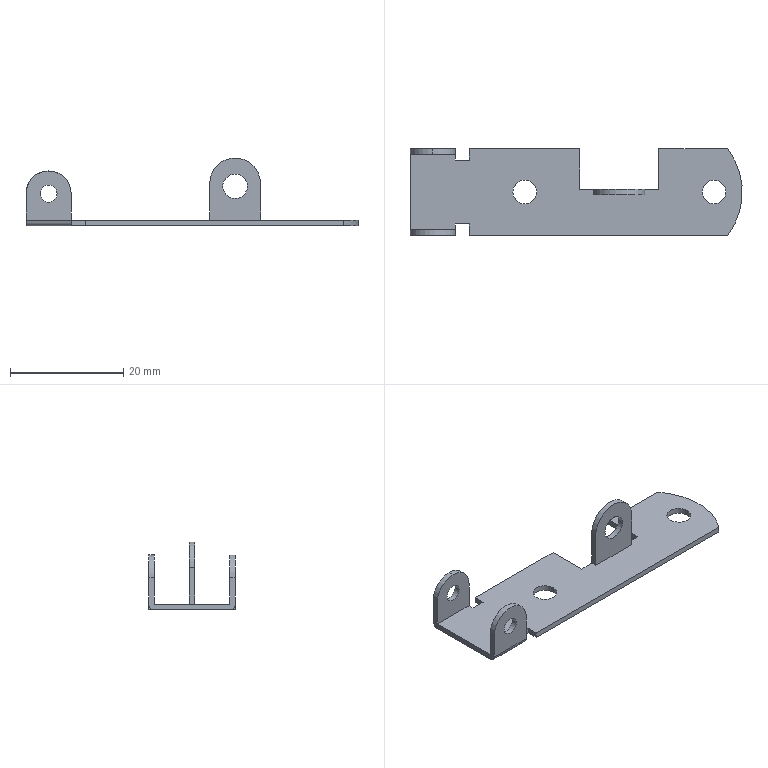Part | SolidWorks | features BaseBody 1 | 1 solid | 44 faces | box 58.8 x 15.3 x 12 mm | volume 930.521 mm3 | plane 26 | cylinder 18 | commonest cylinder face diameters 3 x4 4.2 x4 2 x3 8 x3 4.35 x2 9 x1
STEP:
#1=CARTESIAN_POINT('',(51.7,0.,0.));
#2=VERTEX_POINT('',#1);
#3=CARTESIAN_POINT('',(55.9,0.,0.));
#4=VERTEX_POINT('',#3);
#5=CARTESIAN_POINT('',(53.8,0.,0.));
#6=DIRECTION('',(0.,0.,-1.));
#7=DIRECTION('',(-1.,0.,0.));
#8=AXIS2_PLACEMENT_3D('',#5,#6,#7);
#9=CIRCLE('',#8,2.1);
#10=EDGE_CURVE('',#2,#4,#9,.T.);
#11=ORIENTED_EDGE('',*,*,#10,.F.);
#12=CARTESIAN_POINT('',(51.7,0.,-1.));
#13=VERTEX_POINT('',#12);
#14=CARTESIAN_POINT('',(51.7,0.,-0.5));
#15=DIRECTION('',(0.,0.,-1.));
#16=VECTOR('',#15,1000.);
#17=LINE('',#14,#16);
#18=EDGE_CURVE('',#2,#13,#17,.T.);
#19=ORIENTED_EDGE('',*,*,#18,.T.);
#20=CARTESIAN_POINT('',(55.9,0.,-1.));
#21=VERTEX_POINT('',#20);
#22=CARTESIAN_POINT('',(53.8,0.,-1.));
#23=DIRECTION('',(0.,0.,-1.));
#24=DIRECTION('',(1.,0.,0.));
#25=AXIS2_PLACEMENT_3D('',#22,#23,#24);
#26=CIRCLE('',#25,2.1);
#27=EDGE_CURVE('',#13,#21,#26,.T.);
#28=ORIENTED_EDGE('',*,*,#27,.T.);
#29=CARTESIAN_POINT('',(55.9,0.,-0.5));
#30=DIRECTION('',(0.,0.,-1.));
#31=VECTOR('',#30,1000.);
#32=LINE('',#29,#31);
#33=EDGE_CURVE('',#4,#21,#32,.T.);
#34=ORIENTED_EDGE('',*,*,#33,.F.);
#35=EDGE_LOOP('',(#11,#19,#28,#34));
#36=FACE_OUTER_BOUND('',#35,.T.);
#37=CARTESIAN_POINT('',(53.8,0.,-0.5));
#38=DIRECTION('',(0.,0.,-1.));
#39=DIRECTION('',(1.,0.,0.));
#40=AXIS2_PLACEMENT_3D('',#37,#38,#39);
#41=CYLINDRICAL_SURFACE('',#40,2.1);
#42=ADVANCED_FACE('',(#36),#41,.F.);
#43=CARTESIAN_POINT('',(18.2,0.,0.));
#44=VERTEX_POINT('',#43);
#45=CARTESIAN_POINT('',(22.4,0.,0.));
#46=VERTEX_POINT('',#45);
#47=CARTESIAN_POINT('',(20.3,0.,0.));
#48=DIRECTION('',(0.,0.,-1.));
#49=DIRECTION('',(-1.,0.,0.));
#50=AXIS2_PLACEMENT_3D('',#47,#48,#49);
#51=CIRCLE('',#50,2.1);
#52=EDGE_CURVE('',#44,#46,#51,.T.);
#53=ORIENTED_EDGE('',*,*,#52,.F.);
#54=CARTESIAN_POINT('',(18.2,0.,-1.));
#55=VERTEX_POINT('',#54);
#56=CARTESIAN_POINT('',(18.2,0.,-0.5));
#57=DIRECTION('',(0.,0.,-1.));
#58=VECTOR('',#57,1000.);
#59=LINE('',#56,#58);
#60=EDGE_CURVE('',#44,#55,#59,.T.);
#61=ORIENTED_EDGE('',*,*,#60,.T.);
#62=CARTESIAN_POINT('',(22.4,0.,-1.));
#63=VERTEX_POINT('',#62);
#64=CARTESIAN_POINT('',(20.3,0.,-1.));
#65=DIRECTION('',(0.,0.,-1.));
#66=DIRECTION('',(-1.,0.,0.));
#67=AXIS2_PLACEMENT_3D('',#64,#65,#66);
#68=CIRCLE('',#67,2.1);
#69=EDGE_CURVE('',#55,#63,#68,.T.);
#70=ORIENTED_EDGE('',*,*,#69,.T.);
#71=CARTESIAN_POINT('',(22.4,0.,-0.5));
#72=DIRECTION('',(0.,0.,-1.));
#73=VECTOR('',#72,1000.);
#74=LINE('',#71,#73);
#75=EDGE_CURVE('',#46,#63,#74,.T.);
#76=ORIENTED_EDGE('',*,*,#75,.F.);
#77=EDGE_LOOP('',(#53,#61,#70,#76));
#78=FACE_OUTER_BOUND('',#77,.T.);
#79=CARTESIAN_POINT('',(20.3,0.,-0.5));
#80=DIRECTION('',(0.,0.,-1.));
#81=DIRECTION('',(1.,0.,0.));
#82=AXIS2_PLACEMENT_3D('',#79,#80,#81);
#83=CYLINDRICAL_SURFACE('',#82,2.1);
#84=ADVANCED_FACE('',(#78),#83,.F.);
#85=CARTESIAN_POINT('',(34.825,0.5,6.));
#86=VERTEX_POINT('',#85);
#87=CARTESIAN_POINT('',(39.175,0.5,6.));
#88=VERTEX_POINT('',#87);
#89=CARTESIAN_POINT('',(37.,0.5,6.));
#90=DIRECTION('',(0.,-1.,0.));
#91=DIRECTION('',(-1.,0.,0.));
#92=AXIS2_PLACEMENT_3D('',#89,#90,#91);
#93=CIRCLE('',#92,2.175);
#94=EDGE_CURVE('',#86,#88,#93,.T.);
#95=ORIENTED_EDGE('',*,*,#94,.F.);
#96=CARTESIAN_POINT('',(34.825,-0.5,6.));
#97=VERTEX_POINT('',#96);
#98=CARTESIAN_POINT('',(34.825,-0.5,6.));
#99=DIRECTION('',(0.,-1.,0.));
#100=VECTOR('',#99,1000.);
#101=LINE('',#98,#100);
#102=EDGE_CURVE('',#86,#97,#101,.T.);
#103=ORIENTED_EDGE('',*,*,#102,.T.);
#104=CARTESIAN_POINT('',(39.175,-0.5,6.));
#105=VERTEX_POINT('',#104);
#106=CARTESIAN_POINT('',(37.,-0.5,6.));
#107=DIRECTION('',(0.,-1.,0.));
#108=DIRECTION('',(1.,0.,0.));
#109=AXIS2_PLACEMENT_3D('',#106,#107,#108);
#110=CIRCLE('',#109,2.175);
#111=EDGE_CURVE('',#97,#105,#110,.T.);
#112=ORIENTED_EDGE('',*,*,#111,.T.);
#113=CARTESIAN_POINT('',(39.175,-0.5,6.));
#114=DIRECTION('',(0.,-1.,0.));
#115=VECTOR('',#114,1000.);
#116=LINE('',#113,#115);
#117=EDGE_CURVE('',#88,#105,#116,.T.);
#118=ORIENTED_EDGE('',*,*,#117,.F.);
#119=EDGE_LOOP('',(#95,#103,#112,#118));
#120=FACE_OUTER_BOUND('',#119,.T.);
#121=CARTESIAN_POINT('',(37.,-0.5,6.));
#122=DIRECTION('',(0.,-1.,0.));
#123=DIRECTION('',(1.,0.,0.));
#124=AXIS2_PLACEMENT_3D('',#121,#122,#123);
#125=CYLINDRICAL_SURFACE('',#124,2.175);
#126=ADVANCED_FACE('',(#120),#125,.F.);
#127=CARTESIAN_POINT('',(0.,6.65,4.7));
#128=VERTEX_POINT('',#127);
#129=CARTESIAN_POINT('',(4.,6.65,8.7));
#130=VERTEX_POINT('',#129);
#131=CARTESIAN_POINT('',(4.,6.65,4.7));
#132=DIRECTION('',(0.,1.,0.));
#133=DIRECTION('',(-1.,0.,0.));
#134=AXIS2_PLACEMENT_3D('',#131,#132,#133);
#135=CIRCLE('',#134,4.);
#136=EDGE_CURVE('',#128,#130,#135,.T.);
#137=ORIENTED_EDGE('',*,*,#136,.T.);
#138=CARTESIAN_POINT('',(4.,7.65,8.7));
#139=VERTEX_POINT('',#138);
#140=CARTESIAN_POINT('',(4.,-27.595,8.7));
#141=DIRECTION('',(0.,1.,0.));
#142=VECTOR('',#141,1000.);
#143=LINE('',#140,#142);
#144=EDGE_CURVE('',#130,#139,#143,.T.);
#145=ORIENTED_EDGE('',*,*,#144,.T.);
#146=CARTESIAN_POINT('',(0.,7.65,4.7));
#147=VERTEX_POINT('',#146);
#148=CARTESIAN_POINT('',(4.,7.65,4.7));
#149=DIRECTION('',(0.,-1.,0.));
#150=DIRECTION('',(1.,0.,0.));
#151=AXIS2_PLACEMENT_3D('',#148,#149,#150);
#152=CIRCLE('',#151,4.);
#153=EDGE_CURVE('',#139,#147,#152,.T.);
#154=ORIENTED_EDGE('',*,*,#153,.T.);
#155=CARTESIAN_POINT('',(0.,6.65,4.7));
#156=DIRECTION('',(0.,1.,0.));
#157=VECTOR('',#156,1000.);
#158=LINE('',#155,#157);
#159=EDGE_CURVE('',#128,#147,#158,.T.);
#160=ORIENTED_EDGE('',*,*,#159,.F.);
#161=EDGE_LOOP('',(#137,#145,#154,#160));
#162=FACE_OUTER_BOUND('',#161,.T.);
#163=CARTESIAN_POINT('',(4.,-27.595,4.7));
#164=DIRECTION('',(0.,1.,0.));
#165=DIRECTION('',(0.,0.,1.));
#166=AXIS2_PLACEMENT_3D('',#163,#164,#165);
#167=CYLINDRICAL_SURFACE('',#166,4.);
#168=ADVANCED_FACE('',(#162),#167,.T.);
#169=CARTESIAN_POINT('',(5.5,-6.65,4.7));
#170=VERTEX_POINT('',#169);
#171=CARTESIAN_POINT('',(2.5,-6.65,4.7));
#172=VERTEX_POINT('',#171);
#173=CARTESIAN_POINT('',(4.,-6.65,4.7));
#174=DIRECTION('',(0.,-1.,0.));
#175=DIRECTION('',(1.,0.,0.));
#176=AXIS2_PLACEMENT_3D('',#173,#174,#175);
#177=CIRCLE('',#176,1.5);
#178=EDGE_CURVE('',#170,#172,#177,.T.);
#179=ORIENTED_EDGE('',*,*,#178,.F.);
#180=CARTESIAN_POINT('',(5.5,-7.65,4.7));
#181=VERTEX_POINT('',#180);
#182=CARTESIAN_POINT('',(5.5,-7.15,4.7));
#183=DIRECTION('',(0.,-1.,0.));
#184=VECTOR('',#183,1000.);
#185=LINE('',#182,#184);
#186=EDGE_CURVE('',#170,#181,#185,.T.);
#187=ORIENTED_EDGE('',*,*,#186,.T.);
#188=CARTESIAN_POINT('',(2.5,-7.65,4.7));
#189=VERTEX_POINT('',#188);
#190=CARTESIAN_POINT('',(4.,-7.65,4.7));
#191=DIRECTION('',(0.,-1.,0.));
#192=DIRECTION('',(1.,0.,0.));
#193=AXIS2_PLACEMENT_3D('',#190,#191,#192);
#194=CIRCLE('',#193,1.5);
#195=EDGE_CURVE('',#181,#189,#194,.T.);
#196=ORIENTED_EDGE('',*,*,#195,.T.);
#197=CARTESIAN_POINT('',(2.5,-7.15,4.7));
#198=DIRECTION('',(0.,-1.,0.));
#199=VECTOR('',#198,1000.);
#200=LINE('',#197,#199);
#201=EDGE_CURVE('',#172,#189,#200,.T.);
#202=ORIENTED_EDGE('',*,*,#201,.F.);
#203=EDGE_LOOP('',(#179,#187,#196,#202));
#204=FACE_OUTER_BOUND('',#203,.T.);
#205=CARTESIAN_POINT('',(4.,-7.15,4.7));
#206=DIRECTION('',(0.,-1.,0.));
#207=DIRECTION('',(-1.,0.,0.));
#208=AXIS2_PLACEMENT_3D('',#205,#206,#207);
#209=CYLINDRICAL_SURFACE('',#208,1.5);
#210=ADVANCED_FACE('',(#204),#209,.F.);
#211=CARTESIAN_POINT('',(5.5,7.65,4.7));
#212=VERTEX_POINT('',#211);
#213=CARTESIAN_POINT('',(2.5,7.65,4.7));
#214=VERTEX_POINT('',#213);
#215=CARTESIAN_POINT('',(4.,7.65,4.7));
#216=DIRECTION('',(0.,-1.,0.));
#217=DIRECTION('',(1.,0.,0.));
#218=AXIS2_PLACEMENT_3D('',#215,#216,#217);
#219=CIRCLE('',#218,1.5);
#220=EDGE_CURVE('',#212,#214,#219,.T.);
#221=ORIENTED_EDGE('',*,*,#220,.F.);
#222=CARTESIAN_POINT('',(5.5,6.65,4.7));
#223=VERTEX_POINT('',#222);
#224=CARTESIAN_POINT('',(5.5,7.15,4.7));
#225=DIRECTION('',(0.,-1.,0.));
#226=VECTOR('',#225,1000.);
#227=LINE('',#224,#226);
#228=EDGE_CURVE('',#212,#223,#227,.T.);
#229=ORIENTED_EDGE('',*,*,#228,.T.);
#230=CARTESIAN_POINT('',(2.5,6.65,4.7));
#231=VERTEX_POINT('',#230);
#232=CARTESIAN_POINT('',(4.,6.65,4.7));
#233=DIRECTION('',(0.,-1.,0.));
#234=DIRECTION('',(1.,0.,0.));
#235=AXIS2_PLACEMENT_3D('',#232,#233,#234);
#236=CIRCLE('',#235,1.5);
#237=EDGE_CURVE('',#223,#231,#236,.T.);
#238=ORIENTED_EDGE('',*,*,#237,.T.);
#239=CARTESIAN_POINT('',(2.5,7.15,4.7));
#240=DIRECTION('',(0.,-1.,0.));
#241=VECTOR('',#240,1000.);
#242=LINE('',#239,#241);
#243=EDGE_CURVE('',#214,#231,#242,.T.);
#244=ORIENTED_EDGE('',*,*,#243,.F.);
#245=EDGE_LOOP('',(#221,#229,#238,#244));
#246=FACE_OUTER_BOUND('',#245,.T.);
#247=CARTESIAN_POINT('',(4.,7.15,4.7));
#248=DIRECTION('',(0.,-1.,0.));
#249=DIRECTION('',(-1.,0.,0.));
#250=AXIS2_PLACEMENT_3D('',#247,#248,#249);
#251=CYLINDRICAL_SURFACE('',#250,1.5);
#252=ADVANCED_FACE('',(#246),#251,.F.);
#253=ORIENTED_EDGE('',*,*,#228,.F.);
#254=CARTESIAN_POINT('',(4.,7.65,4.7));
#255=DIRECTION('',(0.,-1.,0.));
#256=DIRECTION('',(1.,0.,0.));
#257=AXIS2_PLACEMENT_3D('',#254,#255,#256);
#258=CIRCLE('',#257,1.5);
#259=EDGE_CURVE('',#214,#212,#258,.T.);
#260=ORIENTED_EDGE('',*,*,#259,.F.);
#261=ORIENTED_EDGE('',*,*,#243,.T.);
#262=CARTESIAN_POINT('',(4.,6.65,4.7));
#263=DIRECTION('',(0.,-1.,0.));
#264=DIRECTION('',(1.,0.,0.));
#265=AXIS2_PLACEMENT_3D('',#262,#263,#264);
#266=CIRCLE('',#265,1.5);
#267=EDGE_CURVE('',#231,#223,#266,.T.);
#268=ORIENTED_EDGE('',*,*,#267,.T.);
#269=EDGE_LOOP('',(#253,#260,#261,#268));
#270=FACE_OUTER_BOUND('',#269,.T.);
#271=CARTESIAN_POINT('',(4.,7.15,4.7));
#272=DIRECTION('',(0.,-1.,0.));
#273=DIRECTION('',(-1.,0.,0.));
#274=AXIS2_PLACEMENT_3D('',#271,#272,#273);
#275=CYLINDRICAL_SURFACE('',#274,1.5);
#276=ADVANCED_FACE('',(#270),#275,.F.);
#277=ORIENTED_EDGE('',*,*,#259,.T.);
#278=ORIENTED_EDGE('',*,*,#220,.T.);
#279=EDGE_LOOP('',(#277,#278));
#280=FACE_BOUND('',#279,.T.);
#281=CARTESIAN_POINT('',(8.,7.65,4.7));
#282=VERTEX_POINT('',#281);
#283=CARTESIAN_POINT('',(8.,7.65,0.));
#284=VERTEX_POINT('',#283);
#285=CARTESIAN_POINT('',(8.,7.65,4.7));
#286=DIRECTION('',(0.,0.,-1.));
#287=VECTOR('',#286,1000.);
#288=LINE('',#285,#287);
#289=EDGE_CURVE('',#282,#284,#288,.T.);
#290=ORIENTED_EDGE('',*,*,#289,.T.);
#291=CARTESIAN_POINT('',(0.,7.65,0.));
#292=VERTEX_POINT('',#291);
#293=CARTESIAN_POINT('',(8.,7.65,0.));
#294=DIRECTION('',(-1.,0.,0.));
#295=VECTOR('',#294,1000.);
#296=LINE('',#293,#295);
#297=EDGE_CURVE('',#284,#292,#296,.T.);
#298=ORIENTED_EDGE('',*,*,#297,.T.);
#299=CARTESIAN_POINT('',(0.,7.65,0.));
#300=DIRECTION('',(0.,0.,1.));
#301=VECTOR('',#300,1000.);
#302=LINE('',#299,#301);
#303=EDGE_CURVE('',#292,#147,#302,.T.);
#304=ORIENTED_EDGE('',*,*,#303,.T.);
#305=ORIENTED_EDGE('',*,*,#153,.F.);
#306=CARTESIAN_POINT('',(4.,7.65,4.7));
#307=DIRECTION('',(0.,-1.,0.));
#308=DIRECTION('',(1.,0.,0.));
#309=AXIS2_PLACEMENT_3D('',#306,#307,#308);
#310=CIRCLE('',#309,4.);
#311=EDGE_CURVE('',#282,#139,#310,.T.);
#312=ORIENTED_EDGE('',*,*,#311,.F.);
#313=EDGE_LOOP('',(#290,#298,#304,#305,#312));
#314=FACE_OUTER_BOUND('',#313,.T.);
#315=CARTESIAN_POINT('',(0.,7.65,-1.));
#316=DIRECTION('',(0.,1.,0.));
#317=DIRECTION('',(1.,0.,0.));
#318=AXIS2_PLACEMENT_3D('',#315,#316,#317);
#319=PLANE('',#318);
#320=ADVANCED_FACE('',(#280,#314),#319,.T.);
#321=CARTESIAN_POINT('',(8.,6.65,-1.));
#322=VERTEX_POINT('',#321);
#323=CARTESIAN_POINT('',(8.,6.65,0.));
#324=DIRECTION('',(-1.,0.,0.));
#325=DIRECTION('',(0.,1.,0.));
#326=AXIS2_PLACEMENT_3D('',#323,#324,#325);
#327=CIRCLE('',#326,1.);
#328=EDGE_CURVE('',#284,#322,#327,.T.);
#329=ORIENTED_EDGE('',*,*,#328,.T.);
#330=CARTESIAN_POINT('',(0.,6.65,-1.));
#331=VERTEX_POINT('',#330);
#332=CARTESIAN_POINT('',(8.,6.65,-1.));
#333=DIRECTION('',(-1.,0.,0.));
#334=VECTOR('',#333,1000.);
#335=LINE('',#332,#334);
#336=EDGE_CURVE('',#322,#331,#335,.T.);
#337=ORIENTED_EDGE('',*,*,#336,.T.);
#338=CARTESIAN_POINT('',(0.,6.65,0.));
#339=DIRECTION('',(-1.,0.,0.));
#340=DIRECTION('',(0.,1.,0.));
#341=AXIS2_PLACEMENT_3D('',#338,#339,#340);
#342=CIRCLE('',#341,1.);
#343=EDGE_CURVE('',#292,#331,#342,.T.);
#344=ORIENTED_EDGE('',*,*,#343,.F.);
#345=ORIENTED_EDGE('',*,*,#297,.F.);
#346=EDGE_LOOP('',(#329,#337,#344,#345));
#347=FACE_OUTER_BOUND('',#346,.T.);
#348=CARTESIAN_POINT('',(8.,6.65,0.));
#349=DIRECTION('',(-1.,0.,0.));
#350=DIRECTION('',(0.,1.,0.));
#351=AXIS2_PLACEMENT_3D('',#348,#349,#350);
#352=CYLINDRICAL_SURFACE('',#351,1.);
#353=ADVANCED_FACE('',(#347),#352,.T.);
#354=CARTESIAN_POINT('',(0.,-7.65,0.));
#355=VERTEX_POINT('',#354);
#356=CARTESIAN_POINT('',(0.,-6.65,-1.));
#357=VERTEX_POINT('',#356);
#358=CARTESIAN_POINT('',(0.,-6.65,0.));
#359=DIRECTION('',(1.,0.,0.));
#360=DIRECTION('',(0.,-1.,0.));
#361=AXIS2_PLACEMENT_3D('',#358,#359,#360);
#362=CIRCLE('',#361,1.);
#363=EDGE_CURVE('',#355,#357,#362,.T.);
#364=ORIENTED_EDGE('',*,*,#363,.T.);
#365=CARTESIAN_POINT('',(8.,-6.65,-1.));
#366=VERTEX_POINT('',#365);
#367=CARTESIAN_POINT('',(0.,-6.65,-1.));
#368=DIRECTION('',(1.,0.,0.));
#369=VECTOR('',#368,1000.);
#370=LINE('',#367,#369);
#371=EDGE_CURVE('',#357,#366,#370,.T.);
#372=ORIENTED_EDGE('',*,*,#371,.T.);
#373=CARTESIAN_POINT('',(8.,-7.65,0.));
#374=VERTEX_POINT('',#373);
#375=CARTESIAN_POINT('',(8.,-6.65,0.));
#376=DIRECTION('',(1.,0.,0.));
#377=DIRECTION('',(0.,-1.,0.));
#378=AXIS2_PLACEMENT_3D('',#375,#376,#377);
#379=CIRCLE('',#378,1.);
#380=EDGE_CURVE('',#374,#366,#379,.T.);
#381=ORIENTED_EDGE('',*,*,#380,.F.);
#382=CARTESIAN_POINT('',(0.,-7.65,0.));
#383=DIRECTION('',(1.,0.,0.));
#384=VECTOR('',#383,1000.);
#385=LINE('',#382,#384);
#386=EDGE_CURVE('',#355,#374,#385,.T.);
#387=ORIENTED_EDGE('',*,*,#386,.F.);
#388=EDGE_LOOP('',(#364,#372,#381,#387));
#389=FACE_OUTER_BOUND('',#388,.T.);
#390=CARTESIAN_POINT('',(0.,-6.65,0.));
#391=DIRECTION('',(1.,0.,0.));
#392=DIRECTION('',(0.,-1.,0.));
#393=AXIS2_PLACEMENT_3D('',#390,#391,#392);
#394=CYLINDRICAL_SURFACE('',#393,1.);
#395=ADVANCED_FACE('',(#389),#394,.T.);
#396=CARTESIAN_POINT('',(44.,7.65,0.));
#397=VERTEX_POINT('',#396);
#398=CARTESIAN_POINT('',(44.,7.65,-1.));
#399=VERTEX_POINT('',#398);
#400=CARTESIAN_POINT('',(44.,7.65,0.));
#401=DIRECTION('',(0.,0.,-1.));
#402=VECTOR('',#401,1000.);
#403=LINE('',#400,#402);
#404=EDGE_CURVE('',#397,#399,#403,.T.);
#405=ORIENTED_EDGE('',*,*,#404,.T.);
#406=CARTESIAN_POINT('',(44.,0.5,-1.));
#407=VERTEX_POINT('',#406);
#408=CARTESIAN_POINT('',(44.,7.65,-1.));
#409=DIRECTION('',(0.,-1.,0.));
#410=VECTOR('',#409,1000.);
#411=LINE('',#408,#410);
#412=EDGE_CURVE('',#399,#407,#411,.T.);
#413=ORIENTED_EDGE('',*,*,#412,.T.);
#414=CARTESIAN_POINT('',(44.,0.5,0.));
#415=VERTEX_POINT('',#414);
#416=CARTESIAN_POINT('',(44.,0.5,0.));
#417=DIRECTION('',(0.,0.,-1.));
#418=VECTOR('',#417,1000.);
#419=LINE('',#416,#418);
#420=EDGE_CURVE('',#415,#407,#419,.T.);
#421=ORIENTED_EDGE('',*,*,#420,.F.);
#422=CARTESIAN_POINT('',(44.,7.65,0.));
#423=DIRECTION('',(0.,-1.,0.));
#424=VECTOR('',#423,1000.);
#425=LINE('',#422,#424);
#426=EDGE_CURVE('',#397,#415,#425,.T.);
#427=ORIENTED_EDGE('',*,*,#426,.F.);
#428=EDGE_LOOP('',(#405,#413,#421,#427));
#429=FACE_OUTER_BOUND('',#428,.T.);
#430=CARTESIAN_POINT('',(44.,4.075,-0.5));
#431=DIRECTION('',(-1.,0.,0.));
#432=DIRECTION('',(0.,0.,1.));
#433=AXIS2_PLACEMENT_3D('',#430,#431,#432);
#434=PLANE('',#433);
#435=ADVANCED_FACE('',(#429),#434,.T.);
#436=CARTESIAN_POINT('',(56.186,7.65,0.));
#437=VERTEX_POINT('',#436);
#438=CARTESIAN_POINT('',(56.186,7.65,0.));
#439=DIRECTION('',(-1.,0.,0.));
#440=VECTOR('',#439,1000.);
#441=LINE('',#438,#440);
#442=EDGE_CURVE('',#437,#397,#441,.T.);
#443=ORIENTED_EDGE('',*,*,#442,.F.);
#444=CARTESIAN_POINT('',(56.186,7.65,-1.));
#445=VERTEX_POINT('',#444);
#446=CARTESIAN_POINT('',(56.186,7.65,0.));
#447=DIRECTION('',(0.,0.,-1.));
#448=VECTOR('',#447,1000.);
#449=LINE('',#446,#448);
#450=EDGE_CURVE('',#437,#445,#449,.T.);
#451=ORIENTED_EDGE('',*,*,#450,.T.);
#452=CARTESIAN_POINT('',(56.186,7.65,-1.));
#453=DIRECTION('',(-1.,0.,0.));
#454=VECTOR('',#453,1000.);
#455=LINE('',#452,#454);
#456=EDGE_CURVE('',#445,#399,#455,.T.);
#457=ORIENTED_EDGE('',*,*,#456,.T.);
#458=ORIENTED_EDGE('',*,*,#404,.F.);
#459=EDGE_LOOP('',(#443,#451,#457,#458));
#460=FACE_OUTER_BOUND('',#459,.T.);
#461=CARTESIAN_POINT('',(28.093,7.65,-0.5));
#462=DIRECTION('',(0.,1.,0.));
#463=DIRECTION('',(1.,0.,0.));
#464=AXIS2_PLACEMENT_3D('',#461,#462,#463);
#465=PLANE('',#464);
#466=ADVANCED_FACE('',(#460),#465,.T.);
#467=CARTESIAN_POINT('',(56.186,-7.65,0.));
#468=VERTEX_POINT('',#467);
#469=CARTESIAN_POINT('',(56.186,-7.65,-1.));
#470=VERTEX_POINT('',#469);
#471=CARTESIAN_POINT('',(56.186,-7.65,0.));
#472=DIRECTION('',(0.,0.,-1.));
#473=VECTOR('',#472,1000.);
#474=LINE('',#471,#473);
#475=EDGE_CURVE('',#468,#470,#474,.T.);
#476=ORIENTED_EDGE('',*,*,#475,.T.);
#477=CARTESIAN_POINT('',(46.3,0.,-1.));
#478=DIRECTION('',(0.,0.,1.));
#479=DIRECTION('',(0.7909,-0.612,0.));
#480=AXIS2_PLACEMENT_3D('',#477,#478,#479);
#481=CIRCLE('',#480,12.5);
#482=EDGE_CURVE('',#470,#445,#481,.T.);
#483=ORIENTED_EDGE('',*,*,#482,.T.);
#484=ORIENTED_EDGE('',*,*,#450,.F.);
#485=CARTESIAN_POINT('',(46.3,0.,0.));
#486=DIRECTION('',(0.,0.,1.));
#487=DIRECTION('',(0.7909,-0.612,0.));
#488=AXIS2_PLACEMENT_3D('',#485,#486,#487);
#489=CIRCLE('',#488,12.5);
#490=EDGE_CURVE('',#468,#437,#489,.T.);
#491=ORIENTED_EDGE('',*,*,#490,.F.);
#492=EDGE_LOOP('',(#476,#483,#484,#491));
#493=FACE_OUTER_BOUND('',#492,.T.);
#494=CARTESIAN_POINT('',(46.3,0.,-0.5));
#495=DIRECTION('',(0.,0.,1.));
#496=DIRECTION('',(0.7909,-0.612,0.));
#497=AXIS2_PLACEMENT_3D('',#494,#495,#496);
#498=CYLINDRICAL_SURFACE('',#497,12.5);
#499=ADVANCED_FACE('',(#493),#498,.T.);
#500=CARTESIAN_POINT('',(10.5,-7.65,-1.));
#501=VERTEX_POINT('',#500);
#502=CARTESIAN_POINT('',(10.5,-7.65,-1.));
#503=DIRECTION('',(1.,0.,0.));
#504=VECTOR('',#503,1000.);
#505=LINE('',#502,#504);
#506=EDGE_CURVE('',#501,#470,#505,.T.);
#507=ORIENTED_EDGE('',*,*,#506,.T.);
#508=ORIENTED_EDGE('',*,*,#475,.F.);
#509=CARTESIAN_POINT('',(10.5,-7.65,0.));
#510=VERTEX_POINT('',#509);
#511=CARTESIAN_POINT('',(10.5,-7.65,0.));
#512=DIRECTION('',(1.,0.,0.));
#513=VECTOR('',#512,1000.);
#514=LINE('',#511,#513);
#515=EDGE_CURVE('',#510,#468,#514,.T.);
#516=ORIENTED_EDGE('',*,*,#515,.F.);
#517=CARTESIAN_POINT('',(10.5,-7.65,0.));
#518=DIRECTION('',(0.,0.,-1.));
#519=VECTOR('',#518,1000.);
#520=LINE('',#517,#519);
#521=EDGE_CURVE('',#510,#501,#520,.T.);
#522=ORIENTED_EDGE('',*,*,#521,.T.);
#523=EDGE_LOOP('',(#507,#508,#516,#522));
#524=FACE_OUTER_BOUND('',#523,.T.);
#525=CARTESIAN_POINT('',(28.093,-7.65,-0.5));
#526=DIRECTION('',(0.,-1.,0.));
#527=DIRECTION('',(0.,0.,-1.));
#528=AXIS2_PLACEMENT_3D('',#525,#526,#527);
#529=PLANE('',#528);
#530=ADVANCED_FACE('',(#524),#529,.T.);
#531=CARTESIAN_POINT('',(10.5,-5.65,0.));
#532=VERTEX_POINT('',#531);
#533=CARTESIAN_POINT('',(10.5,-5.65,-1.));
#534=VERTEX_POINT('',#533);
#535=CARTESIAN_POINT('',(10.5,-5.65,0.));
#536=DIRECTION('',(0.,0.,-1.));
#537=VECTOR('',#536,1000.);
#538=LINE('',#535,#537);
#539=EDGE_CURVE('',#532,#534,#538,.T.);
#540=ORIENTED_EDGE('',*,*,#539,.T.);
#541=CARTESIAN_POINT('',(10.5,-7.65,-1.));
#542=DIRECTION('',(0.,1.,0.));
#543=VECTOR('',#542,1000.);
#544=LINE('',#541,#543);
#545=EDGE_CURVE('',#501,#534,#544,.T.);
#546=ORIENTED_EDGE('',*,*,#545,.F.);
#547=ORIENTED_EDGE('',*,*,#521,.F.);
#548=CARTESIAN_POINT('',(10.5,-7.65,0.));
#549=DIRECTION('',(0.,1.,0.));
#550=VECTOR('',#549,1000.);
#551=LINE('',#548,#550);
#552=EDGE_CURVE('',#510,#532,#551,.T.);
#553=ORIENTED_EDGE('',*,*,#552,.T.);
#554=EDGE_LOOP('',(#540,#546,#547,#553));
#555=FACE_OUTER_BOUND('',#554,.T.);
#556=CARTESIAN_POINT('',(10.5,-6.65,-0.5));
#557=DIRECTION('',(1.,0.,0.));
#558=DIRECTION('',(0.,1.,0.));
#559=AXIS2_PLACEMENT_3D('',#556,#557,#558);
#560=PLANE('',#559);
#561=ADVANCED_FACE('',(#555),#560,.F.);
#562=CARTESIAN_POINT('',(8.,-5.65,0.));
#563=VERTEX_POINT('',#562);
#564=CARTESIAN_POINT('',(8.,-5.65,-1.));
#565=VERTEX_POINT('',#564);
#566=CARTESIAN_POINT('',(8.,-5.65,0.));
#567=DIRECTION('',(0.,0.,-1.));
#568=VECTOR('',#567,1000.);
#569=LINE('',#566,#568);
#570=EDGE_CURVE('',#563,#565,#569,.T.);
#571=ORIENTED_EDGE('',*,*,#570,.T.);
#572=CARTESIAN_POINT('',(10.5,-5.65,-1.));
#573=DIRECTION('',(-1.,0.,0.));
#574=VECTOR('',#573,1000.);
#575=LINE('',#572,#574);
#576=EDGE_CURVE('',#534,#565,#575,.T.);
#577=ORIENTED_EDGE('',*,*,#576,.F.);
#578=ORIENTED_EDGE('',*,*,#539,.F.);
#579=CARTESIAN_POINT('',(10.5,-5.65,0.));
#580=DIRECTION('',(-1.,0.,0.));
#581=VECTOR('',#580,1000.);
#582=LINE('',#579,#581);
#583=EDGE_CURVE('',#532,#563,#582,.T.);
#584=ORIENTED_EDGE('',*,*,#583,.T.);
#585=EDGE_LOOP('',(#571,#577,#578,#584));
#586=FACE_OUTER_BOUND('',#585,.T.);
#587=CARTESIAN_POINT('',(9.25,-5.65,-0.5));
#588=DIRECTION('',(0.,1.,0.));
#589=DIRECTION('',(1.,0.,0.));
#590=AXIS2_PLACEMENT_3D('',#587,#588,#589);
#591=PLANE('',#590);
#592=ADVANCED_FACE('',(#586),#591,.F.);
#593=ORIENTED_EDGE('',*,*,#186,.F.);
#594=CARTESIAN_POINT('',(4.,-6.65,4.7));
#595=DIRECTION('',(0.,-1.,0.));
#596=DIRECTION('',(1.,0.,0.));
#597=AXIS2_PLACEMENT_3D('',#594,#595,#596);
#598=CIRCLE('',#597,1.5);
#599=EDGE_CURVE('',#172,#170,#598,.T.);
#600=ORIENTED_EDGE('',*,*,#599,.F.);
#601=ORIENTED_EDGE('',*,*,#201,.T.);
#602=CARTESIAN_POINT('',(4.,-7.65,4.7));
#603=DIRECTION('',(0.,-1.,0.));
#604=DIRECTION('',(1.,0.,0.));
#605=AXIS2_PLACEMENT_3D('',#602,#603,#604);
#606=CIRCLE('',#605,1.5);
#607=EDGE_CURVE('',#189,#181,#606,.T.);
#608=ORIENTED_EDGE('',*,*,#607,.T.);
#609=EDGE_LOOP('',(#593,#600,#601,#608));
#610=FACE_OUTER_BOUND('',#609,.T.);
#611=CARTESIAN_POINT('',(4.,-7.15,4.7));
#612=DIRECTION('',(0.,-1.,0.));
#613=DIRECTION('',(-1.,0.,0.));
#614=AXIS2_PLACEMENT_3D('',#611,#612,#613);
#615=CYLINDRICAL_SURFACE('',#614,1.5);
#616=ADVANCED_FACE('',(#610),#615,.F.);
#617=ORIENTED_EDGE('',*,*,#599,.T.);
#618=ORIENTED_EDGE('',*,*,#178,.T.);
#619=EDGE_LOOP('',(#617,#618));
#620=FACE_BOUND('',#619,.T.);
#621=CARTESIAN_POINT('',(0.,-6.65,4.7));
#622=VERTEX_POINT('',#621);
#623=CARTESIAN_POINT('',(0.,-6.65,0.));
#624=VERTEX_POINT('',#623);
#625=CARTESIAN_POINT('',(0.,-6.65,4.7));
#626=DIRECTION('',(0.,0.,-1.));
#627=VECTOR('',#626,1000.);
#628=LINE('',#625,#627);
#629=EDGE_CURVE('',#622,#624,#628,.T.);
#630=ORIENTED_EDGE('',*,*,#629,.F.);
#631=CARTESIAN_POINT('',(8.,-6.65,4.7));
#632=VERTEX_POINT('',#631);
#633=CARTESIAN_POINT('',(4.,-6.65,4.7));
#634=DIRECTION('',(0.,-1.,0.));
#635=DIRECTION('',(1.,0.,0.));
#636=AXIS2_PLACEMENT_3D('',#633,#634,#635);
#637=CIRCLE('',#636,4.);
#638=EDGE_CURVE('',#632,#622,#637,.T.);
#639=ORIENTED_EDGE('',*,*,#638,.F.);
#640=CARTESIAN_POINT('',(8.,-6.65,0.));
#641=VERTEX_POINT('',#640);
#642=CARTESIAN_POINT('',(8.,-6.65,0.));
#643=DIRECTION('',(0.,0.,1.));
#644=VECTOR('',#643,1000.);
#645=LINE('',#642,#644);
#646=EDGE_CURVE('',#641,#632,#645,.T.);
#647=ORIENTED_EDGE('',*,*,#646,.F.);
#648=CARTESIAN_POINT('',(0.,-6.65,0.));
#649=DIRECTION('',(1.,0.,0.));
#650=VECTOR('',#649,1000.);
#651=LINE('',#648,#650);
#652=EDGE_CURVE('',#624,#641,#651,.T.);
#653=ORIENTED_EDGE('',*,*,#652,.F.);
#654=EDGE_LOOP('',(#630,#639,#647,#653));
#655=FACE_OUTER_BOUND('',#654,.T.);
#656=CARTESIAN_POINT('',(8.,-6.65,-1.));
#657=DIRECTION('',(0.,-1.,0.));
#658=DIRECTION('',(0.,0.,-1.));
#659=AXIS2_PLACEMENT_3D('',#656,#657,#658);
#660=PLANE('',#659);
#661=ADVANCED_FACE('',(#620,#655),#660,.F.);
#662=CARTESIAN_POINT('',(8.,-7.65,4.7));
#663=VERTEX_POINT('',#662);
#664=CARTESIAN_POINT('',(8.,-7.65,0.));
#665=DIRECTION('',(0.,0.,1.));
#666=VECTOR('',#665,1000.);
#667=LINE('',#664,#666);
#668=EDGE_CURVE('',#374,#663,#667,.T.);
#669=ORIENTED_EDGE('',*,*,#668,.F.);
#670=ORIENTED_EDGE('',*,*,#380,.T.);
#671=CARTESIAN_POINT('',(8.,-6.65,-1.));
#672=DIRECTION('',(0.,1.,0.));
#673=VECTOR('',#672,1000.);
#674=LINE('',#671,#673);
#675=EDGE_CURVE('',#366,#565,#674,.T.);
#676=ORIENTED_EDGE('',*,*,#675,.T.);
#677=ORIENTED_EDGE('',*,*,#570,.F.);
#678=CARTESIAN_POINT('',(8.,-6.65,0.));
#679=DIRECTION('',(0.,1.,0.));
#680=VECTOR('',#679,1000.);
#681=LINE('',#678,#680);
#682=EDGE_CURVE('',#641,#563,#681,.T.);
#683=ORIENTED_EDGE('',*,*,#682,.F.);
#684=ORIENTED_EDGE('',*,*,#646,.T.);
#685=CARTESIAN_POINT('',(8.,-6.65,4.7));
#686=DIRECTION('',(0.,-1.,0.));
#687=VECTOR('',#686,1000.);
#688=LINE('',#685,#687);
#689=EDGE_CURVE('',#632,#663,#688,.T.);
#690=ORIENTED_EDGE('',*,*,#689,.T.);
#691=EDGE_LOOP('',(#669,#670,#676,#677,#683,#684,#690));
#692=FACE_OUTER_BOUND('',#691,.T.);
#693=CARTESIAN_POINT('',(8.,-7.15,4.35));
#694=DIRECTION('',(1.,0.,0.));
#695=DIRECTION('',(0.,1.,0.));
#696=AXIS2_PLACEMENT_3D('',#693,#694,#695);
#697=PLANE('',#696);
#698=ADVANCED_FACE('',(#692),#697,.T.);
#699=ORIENTED_EDGE('',*,*,#607,.F.);
#700=ORIENTED_EDGE('',*,*,#195,.F.);
#701=EDGE_LOOP('',(#699,#700));
#702=FACE_BOUND('',#701,.T.);
#703=CARTESIAN_POINT('',(0.,-7.65,4.7));
#704=VERTEX_POINT('',#703);
#705=CARTESIAN_POINT('',(0.,-7.65,4.7));
#706=DIRECTION('',(0.,0.,-1.));
#707=VECTOR('',#706,1000.);
#708=LINE('',#705,#707);
#709=EDGE_CURVE('',#704,#355,#708,.T.);
#710=ORIENTED_EDGE('',*,*,#709,.T.);
#711=ORIENTED_EDGE('',*,*,#386,.T.);
#712=ORIENTED_EDGE('',*,*,#668,.T.);
#713=CARTESIAN_POINT('',(4.,-7.65,4.7));
#714=DIRECTION('',(0.,1.,0.));
#715=DIRECTION('',(-1.,0.,0.));
#716=AXIS2_PLACEMENT_3D('',#713,#714,#715);
#717=CIRCLE('',#716,4.);
#718=EDGE_CURVE('',#704,#663,#717,.T.);
#719=ORIENTED_EDGE('',*,*,#718,.F.);
#720=EDGE_LOOP('',(#710,#711,#712,#719));
#721=FACE_OUTER_BOUND('',#720,.T.);
#722=CARTESIAN_POINT('',(8.,-7.65,-1.));
#723=DIRECTION('',(0.,-1.,0.));
#724=DIRECTION('',(0.,0.,-1.));
#725=AXIS2_PLACEMENT_3D('',#722,#723,#724);
#726=PLANE('',#725);
#727=ADVANCED_FACE('',(#702,#721),#726,.T.);
#728=ORIENTED_EDGE('',*,*,#689,.F.);
#729=ORIENTED_EDGE('',*,*,#638,.T.);
#730=CARTESIAN_POINT('',(0.,-6.65,4.7));
#731=DIRECTION('',(0.,-1.,0.));
#732=VECTOR('',#731,1000.);
#733=LINE('',#730,#732);
#734=EDGE_CURVE('',#622,#704,#733,.T.);
#735=ORIENTED_EDGE('',*,*,#734,.T.);
#736=ORIENTED_EDGE('',*,*,#718,.T.);
#737=EDGE_LOOP('',(#728,#729,#735,#736));
#738=FACE_OUTER_BOUND('',#737,.T.);
#739=CARTESIAN_POINT('',(4.,27.595,4.7));
#740=DIRECTION('',(0.,-1.,0.));
#741=DIRECTION('',(1.,0.,0.));
#742=AXIS2_PLACEMENT_3D('',#739,#740,#741);
#743=CYLINDRICAL_SURFACE('',#742,4.);
#744=ADVANCED_FACE('',(#738),#743,.T.);
#745=ORIENTED_EDGE('',*,*,#303,.F.);
#746=ORIENTED_EDGE('',*,*,#343,.T.);
#747=CARTESIAN_POINT('',(0.,6.65,-1.));
#748=DIRECTION('',(0.,-1.,0.));
#749=VECTOR('',#748,1000.);
#750=LINE('',#747,#749);
#751=EDGE_CURVE('',#331,#357,#750,.T.);
#752=ORIENTED_EDGE('',*,*,#751,.T.);
#753=ORIENTED_EDGE('',*,*,#363,.F.);
#754=ORIENTED_EDGE('',*,*,#709,.F.);
#755=ORIENTED_EDGE('',*,*,#734,.F.);
#756=ORIENTED_EDGE('',*,*,#629,.T.);
#757=CARTESIAN_POINT('',(0.,6.65,0.));
#758=VERTEX_POINT('',#757);
#759=CARTESIAN_POINT('',(0.,6.65,0.));
#760=DIRECTION('',(0.,-1.,0.));
#761=VECTOR('',#760,1000.);
#762=LINE('',#759,#761);
#763=EDGE_CURVE('',#758,#624,#762,.T.);
#764=ORIENTED_EDGE('',*,*,#763,.F.);
#765=CARTESIAN_POINT('',(0.,6.65,0.));
#766=DIRECTION('',(0.,0.,1.));
#767=VECTOR('',#766,1000.);
#768=LINE('',#765,#767);
#769=EDGE_CURVE('',#758,#128,#768,.T.);
#770=ORIENTED_EDGE('',*,*,#769,.T.);
#771=ORIENTED_EDGE('',*,*,#159,.T.);
#772=EDGE_LOOP('',(#745,#746,#752,#753,#754,#755,#756,#764,#770,#771));
#773=FACE_OUTER_BOUND('',#772,.T.);
#774=CARTESIAN_POINT('',(0.,7.15,4.35));
#775=DIRECTION('',(-1.,0.,0.));
#776=DIRECTION('',(0.,0.,1.));
#777=AXIS2_PLACEMENT_3D('',#774,#775,#776);
#778=PLANE('',#777);
#779=ADVANCED_FACE('',(#773),#778,.T.);
#780=ORIENTED_EDGE('',*,*,#267,.F.);
#781=ORIENTED_EDGE('',*,*,#237,.F.);
#782=EDGE_LOOP('',(#780,#781));
#783=FACE_BOUND('',#782,.T.);
#784=CARTESIAN_POINT('',(8.,6.65,4.7));
#785=VERTEX_POINT('',#784);
#786=CARTESIAN_POINT('',(8.,6.65,0.));
#787=VERTEX_POINT('',#786);
#788=CARTESIAN_POINT('',(8.,6.65,4.7));
#789=DIRECTION('',(0.,0.,-1.));
#790=VECTOR('',#789,1000.);
#791=LINE('',#788,#790);
#792=EDGE_CURVE('',#785,#787,#791,.T.);
#793=ORIENTED_EDGE('',*,*,#792,.F.);
#794=CARTESIAN_POINT('',(4.,6.65,4.7));
#795=DIRECTION('',(0.,1.,0.));
#796=DIRECTION('',(-1.,0.,0.));
#797=AXIS2_PLACEMENT_3D('',#794,#795,#796);
#798=CIRCLE('',#797,4.);
#799=EDGE_CURVE('',#130,#785,#798,.T.);
#800=ORIENTED_EDGE('',*,*,#799,.F.);
#801=ORIENTED_EDGE('',*,*,#136,.F.);
#802=ORIENTED_EDGE('',*,*,#769,.F.);
#803=CARTESIAN_POINT('',(8.,6.65,0.));
#804=DIRECTION('',(-1.,0.,0.));
#805=VECTOR('',#804,1000.);
#806=LINE('',#803,#805);
#807=EDGE_CURVE('',#787,#758,#806,.T.);
#808=ORIENTED_EDGE('',*,*,#807,.F.);
#809=EDGE_LOOP('',(#793,#800,#801,#802,#808));
#810=FACE_OUTER_BOUND('',#809,.T.);
#811=CARTESIAN_POINT('',(0.,6.65,-1.));
#812=DIRECTION('',(0.,1.,0.));
#813=DIRECTION('',(1.,0.,0.));
#814=AXIS2_PLACEMENT_3D('',#811,#812,#813);
#815=PLANE('',#814);
#816=ADVANCED_FACE('',(#783,#810),#815,.F.);
#817=ORIENTED_EDGE('',*,*,#144,.F.);
#818=ORIENTED_EDGE('',*,*,#799,.T.);
#819=CARTESIAN_POINT('',(8.,6.65,4.7));
#820=DIRECTION('',(0.,1.,0.));
#821=VECTOR('',#820,1000.);
#822=LINE('',#819,#821);
#823=EDGE_CURVE('',#785,#282,#822,.T.);
#824=ORIENTED_EDGE('',*,*,#823,.T.);
#825=ORIENTED_EDGE('',*,*,#311,.T.);
#826=EDGE_LOOP('',(#817,#818,#824,#825));
#827=FACE_OUTER_BOUND('',#826,.T.);
#828=CARTESIAN_POINT('',(4.,-27.595,4.7));
#829=DIRECTION('',(0.,1.,0.));
#830=DIRECTION('',(0.,0.,1.));
#831=AXIS2_PLACEMENT_3D('',#828,#829,#830);
#832=CYLINDRICAL_SURFACE('',#831,4.);
#833=ADVANCED_FACE('',(#827),#832,.T.);
#834=CARTESIAN_POINT('',(8.,5.65,0.));
#835=VERTEX_POINT('',#834);
#836=CARTESIAN_POINT('',(8.,5.65,-1.));
#837=VERTEX_POINT('',#836);
#838=CARTESIAN_POINT('',(8.,5.65,0.));
#839=DIRECTION('',(0.,0.,-1.));
#840=VECTOR('',#839,1000.);
#841=LINE('',#838,#840);
#842=EDGE_CURVE('',#835,#837,#841,.T.);
#843=ORIENTED_EDGE('',*,*,#842,.T.);
#844=CARTESIAN_POINT('',(8.,6.65,-1.));
#845=DIRECTION('',(0.,-1.,0.));
#846=VECTOR('',#845,1000.);
#847=LINE('',#844,#846);
#848=EDGE_CURVE('',#322,#837,#847,.T.);
#849=ORIENTED_EDGE('',*,*,#848,.F.);
#850=ORIENTED_EDGE('',*,*,#328,.F.);
#851=ORIENTED_EDGE('',*,*,#289,.F.);
#852=ORIENTED_EDGE('',*,*,#823,.F.);
#853=ORIENTED_EDGE('',*,*,#792,.T.);
#854=CARTESIAN_POINT('',(8.,6.65,0.));
#855=DIRECTION('',(0.,-1.,0.));
#856=VECTOR('',#855,1000.);
#857=LINE('',#854,#856);
#858=EDGE_CURVE('',#787,#835,#857,.T.);
#859=ORIENTED_EDGE('',*,*,#858,.T.);
#860=EDGE_LOOP('',(#843,#849,#850,#851,#852,#853,#859));
#861=FACE_OUTER_BOUND('',#860,.T.);
#862=CARTESIAN_POINT('',(8.,6.65,-0.5));
#863=DIRECTION('',(-1.,0.,0.));
#864=DIRECTION('',(0.,0.,1.));
#865=AXIS2_PLACEMENT_3D('',#862,#863,#864);
#866=PLANE('',#865);
#867=ADVANCED_FACE('',(#861),#866,.F.);
#868=CARTESIAN_POINT('',(10.5,5.65,0.));
#869=VERTEX_POINT('',#868);
#870=CARTESIAN_POINT('',(10.5,5.65,-1.));
#871=VERTEX_POINT('',#870);
#872=CARTESIAN_POINT('',(10.5,5.65,0.));
#873=DIRECTION('',(0.,0.,-1.));
#874=VECTOR('',#873,1000.);
#875=LINE('',#872,#874);
#876=EDGE_CURVE('',#869,#871,#875,.T.);
#877=ORIENTED_EDGE('',*,*,#876,.T.);
#878=CARTESIAN_POINT('',(8.,5.65,-1.));
#879=DIRECTION('',(1.,0.,0.));
#880=VECTOR('',#879,1000.);
#881=LINE('',#878,#880);
#882=EDGE_CURVE('',#837,#871,#881,.T.);
#883=ORIENTED_EDGE('',*,*,#882,.F.);
#884=ORIENTED_EDGE('',*,*,#842,.F.);
#885=CARTESIAN_POINT('',(8.,5.65,0.));
#886=DIRECTION('',(1.,0.,0.));
#887=VECTOR('',#886,1000.);
#888=LINE('',#885,#887);
#889=EDGE_CURVE('',#835,#869,#888,.T.);
#890=ORIENTED_EDGE('',*,*,#889,.T.);
#891=EDGE_LOOP('',(#877,#883,#884,#890));
#892=FACE_OUTER_BOUND('',#891,.T.);
#893=CARTESIAN_POINT('',(9.25,5.65,-0.5));
#894=DIRECTION('',(0.,-1.,0.));
#895=DIRECTION('',(0.,0.,-1.));
#896=AXIS2_PLACEMENT_3D('',#893,#894,#895);
#897=PLANE('',#896);
#898=ADVANCED_FACE('',(#892),#897,.F.);
#899=CARTESIAN_POINT('',(10.5,7.65,0.));
#900=VERTEX_POINT('',#899);
#901=CARTESIAN_POINT('',(10.5,7.65,-1.));
#902=VERTEX_POINT('',#901);
#903=CARTESIAN_POINT('',(10.5,7.65,0.));
#904=DIRECTION('',(0.,0.,-1.));
#905=VECTOR('',#904,1000.);
#906=LINE('',#903,#905);
#907=EDGE_CURVE('',#900,#902,#906,.T.);
#908=ORIENTED_EDGE('',*,*,#907,.T.);
#909=CARTESIAN_POINT('',(10.5,7.65,-1.));
#910=DIRECTION('',(0.,-1.,0.));
#911=VECTOR('',#910,1000.);
#912=LINE('',#909,#911);
#913=EDGE_CURVE('',#902,#871,#912,.T.);
#914=ORIENTED_EDGE('',*,*,#913,.T.);
#915=ORIENTED_EDGE('',*,*,#876,.F.);
#916=CARTESIAN_POINT('',(10.5,7.65,0.));
#917=DIRECTION('',(0.,-1.,0.));
#918=VECTOR('',#917,1000.);
#919=LINE('',#916,#918);
#920=EDGE_CURVE('',#900,#869,#919,.T.);
#921=ORIENTED_EDGE('',*,*,#920,.F.);
#922=EDGE_LOOP('',(#908,#914,#915,#921));
#923=FACE_OUTER_BOUND('',#922,.T.);
#924=CARTESIAN_POINT('',(10.5,6.65,-0.5));
#925=DIRECTION('',(-1.,0.,0.));
#926=DIRECTION('',(0.,0.,1.));
#927=AXIS2_PLACEMENT_3D('',#924,#925,#926);
#928=PLANE('',#927);
#929=ADVANCED_FACE('',(#923),#928,.T.);
#930=CARTESIAN_POINT('',(30.,7.65,-1.));
#931=VERTEX_POINT('',#930);
#932=CARTESIAN_POINT('',(30.,7.65,-1.));
#933=DIRECTION('',(-1.,0.,0.));
#934=VECTOR('',#933,1000.);
#935=LINE('',#932,#934);
#936=EDGE_CURVE('',#931,#902,#935,.T.);
#937=ORIENTED_EDGE('',*,*,#936,.T.);
#938=ORIENTED_EDGE('',*,*,#907,.F.);
#939=CARTESIAN_POINT('',(30.,7.65,0.));
#940=VERTEX_POINT('',#939);
#941=CARTESIAN_POINT('',(30.,7.65,0.));
#942=DIRECTION('',(-1.,0.,0.));
#943=VECTOR('',#942,1000.);
#944=LINE('',#941,#943);
#945=EDGE_CURVE('',#940,#900,#944,.T.);
#946=ORIENTED_EDGE('',*,*,#945,.F.);
#947=CARTESIAN_POINT('',(30.,7.65,0.));
#948=DIRECTION('',(0.,0.,-1.));
#949=VECTOR('',#948,1000.);
#950=LINE('',#947,#949);
#951=EDGE_CURVE('',#940,#931,#950,.T.);
#952=ORIENTED_EDGE('',*,*,#951,.T.);
#953=EDGE_LOOP('',(#937,#938,#946,#952));
#954=FACE_OUTER_BOUND('',#953,.T.);
#955=CARTESIAN_POINT('',(28.093,7.65,-0.5));
#956=DIRECTION('',(0.,1.,0.));
#957=DIRECTION('',(1.,0.,0.));
#958=AXIS2_PLACEMENT_3D('',#955,#956,#957);
#959=PLANE('',#958);
#960=ADVANCED_FACE('',(#954),#959,.T.);
#961=CARTESIAN_POINT('',(30.,0.5,0.));
#962=VERTEX_POINT('',#961);
#963=CARTESIAN_POINT('',(30.,0.5,-1.));
#964=VERTEX_POINT('',#963);
#965=CARTESIAN_POINT('',(30.,0.5,0.));
#966=DIRECTION('',(0.,0.,-1.));
#967=VECTOR('',#966,1000.);
#968=LINE('',#965,#967);
#969=EDGE_CURVE('',#962,#964,#968,.T.);
#970=ORIENTED_EDGE('',*,*,#969,.T.);
#971=CARTESIAN_POINT('',(30.,7.65,-1.));
#972=DIRECTION('',(0.,-1.,0.));
#973=VECTOR('',#972,1000.);
#974=LINE('',#971,#973);
#975=EDGE_CURVE('',#931,#964,#974,.T.);
#976=ORIENTED_EDGE('',*,*,#975,.F.);
#977=ORIENTED_EDGE('',*,*,#951,.F.);
#978=CARTESIAN_POINT('',(30.,7.65,0.));
#979=DIRECTION('',(0.,-1.,0.));
#980=VECTOR('',#979,1000.);
#981=LINE('',#978,#980);
#982=EDGE_CURVE('',#940,#962,#981,.T.);
#983=ORIENTED_EDGE('',*,*,#982,.T.);
#984=EDGE_LOOP('',(#970,#976,#977,#983));
#985=FACE_OUTER_BOUND('',#984,.T.);
#986=CARTESIAN_POINT('',(30.,4.075,-0.5));
#987=DIRECTION('',(-1.,0.,0.));
#988=DIRECTION('',(0.,0.,1.));
#989=AXIS2_PLACEMENT_3D('',#986,#987,#988);
#990=PLANE('',#989);
#991=ADVANCED_FACE('',(#985),#990,.F.);
#992=CARTESIAN_POINT('',(41.5,0.5,0.));
#993=VERTEX_POINT('',#992);
#994=CARTESIAN_POINT('',(41.5,0.5,-1.));
#995=VERTEX_POINT('',#994);
#996=CARTESIAN_POINT('',(41.5,0.5,0.));
#997=DIRECTION('',(0.,0.,-1.));
#998=VECTOR('',#997,1000.);
#999=LINE('',#996,#998);
#1000=EDGE_CURVE('',#993,#995,#999,.T.);
#1001=ORIENTED_EDGE('',*,*,#1000,.T.);
#1002=CARTESIAN_POINT('',(41.5,-0.5,-1.));
#1003=VERTEX_POINT('',#1002);
#1004=CARTESIAN_POINT('',(41.5,-0.5,-1.));
#1005=DIRECTION('',(0.,1.,0.));
#1006=VECTOR('',#1005,1000.);
#1007=LINE('',#1004,#1006);
#1008=EDGE_CURVE('',#1003,#995,#1007,.T.);
#1009=ORIENTED_EDGE('',*,*,#1008,.F.);
#1010=CARTESIAN_POINT('',(41.5,-0.5,0.));
#1011=VERTEX_POINT('',#1010);
#1012=CARTESIAN_POINT('',(41.5,-0.5,-1.));
#1013=DIRECTION('',(0.,0.,1.));
#1014=VECTOR('',#1013,1000.);
#1015=LINE('',#1012,#1014);
#1016=EDGE_CURVE('',#1003,#1011,#1015,.T.);
#1017=ORIENTED_EDGE('',*,*,#1016,.T.);
#1018=CARTESIAN_POINT('',(41.5,-0.5,0.));
#1019=DIRECTION('',(0.,1.,0.));
#1020=VECTOR('',#1019,1000.);
#1021=LINE('',#1018,#1020);
#1022=EDGE_CURVE('',#1011,#993,#1021,.T.);
#1023=ORIENTED_EDGE('',*,*,#1022,.T.);
#1024=EDGE_LOOP('',(#1001,#1009,#1017,#1023));
#1025=FACE_OUTER_BOUND('',#1024,.T.);
#1026=CARTESIAN_POINT('',(41.5,0.,-0.5));
#1027=DIRECTION('',(1.,0.,0.));
#1028=DIRECTION('',(0.,1.,0.));
#1029=AXIS2_PLACEMENT_3D('',#1026,#1027,#1028);
#1030=PLANE('',#1029);
#1031=ADVANCED_FACE('',(#1025),#1030,.F.);
#1032=CARTESIAN_POINT('',(41.5,-0.5,6.5));
#1033=VERTEX_POINT('',#1032);
#1034=CARTESIAN_POINT('',(41.5,-0.5,6.5));
#1035=DIRECTION('',(0.,0.,-1.));
#1036=VECTOR('',#1035,1000.);
#1037=LINE('',#1034,#1036);
#1038=EDGE_CURVE('',#1033,#1011,#1037,.T.);
#1039=ORIENTED_EDGE('',*,*,#1038,.T.);
#1040=ORIENTED_EDGE('',*,*,#1016,.F.);
#1041=CARTESIAN_POINT('',(41.5,0.5,0.));
#1042=VERTEX_POINT('',#1041);
#1043=CARTESIAN_POINT('',(41.5,-0.5,0.));
#1044=DIRECTION('',(-1.,0.,0.));
#1045=DIRECTION('',(0.,1.,0.));
#1046=AXIS2_PLACEMENT_3D('',#1043,#1044,#1045);
#1047=CIRCLE('',#1046,1.);
#1048=EDGE_CURVE('',#1042,#1003,#1047,.T.);
#1049=ORIENTED_EDGE('',*,*,#1048,.F.);
#1050=CARTESIAN_POINT('',(41.5,0.5,6.5));
#1051=VERTEX_POINT('',#1050);
#1052=CARTESIAN_POINT('',(41.5,0.5,6.5));
#1053=DIRECTION('',(0.,0.,-1.));
#1054=VECTOR('',#1053,1000.);
#1055=LINE('',#1052,#1054);
#1056=EDGE_CURVE('',#1051,#1042,#1055,.T.);
#1057=ORIENTED_EDGE('',*,*,#1056,.F.);
#1058=CARTESIAN_POINT('',(41.5,-0.5,6.5));
#1059=DIRECTION('',(0.,1.,0.));
#1060=VECTOR('',#1059,1000.);
#1061=LINE('',#1058,#1060);
#1062=EDGE_CURVE('',#1033,#1051,#1061,.T.);
#1063=ORIENTED_EDGE('',*,*,#1062,.F.);
#1064=EDGE_LOOP('',(#1039,#1040,#1049,#1057,#1063));
#1065=FACE_OUTER_BOUND('',#1064,.T.);
#1066=CARTESIAN_POINT('',(41.5,0.,5.5));
#1067=DIRECTION('',(1.,0.,0.));
#1068=DIRECTION('',(0.,1.,0.));
#1069=AXIS2_PLACEMENT_3D('',#1066,#1067,#1068);
#1070=PLANE('',#1069);
#1071=ADVANCED_FACE('',(#1065),#1070,.T.);
#1072=CARTESIAN_POINT('',(32.5,-0.5,6.5));
#1073=VERTEX_POINT('',#1072);
#1074=CARTESIAN_POINT('',(32.5,0.5,6.5));
#1075=VERTEX_POINT('',#1074);
#1076=CARTESIAN_POINT('',(32.5,-0.5,6.5));
#1077=DIRECTION('',(0.,1.,0.));
#1078=VECTOR('',#1077,1000.);
#1079=LINE('',#1076,#1078);
#1080=EDGE_CURVE('',#1073,#1075,#1079,.T.);
#1081=ORIENTED_EDGE('',*,*,#1080,.F.);
#1082=CARTESIAN_POINT('',(37.,-0.5,6.5));
#1083=DIRECTION('',(0.,1.,0.));
#1084=DIRECTION('',(-1.,0.,0.));
#1085=AXIS2_PLACEMENT_3D('',#1082,#1083,#1084);
#1086=CIRCLE('',#1085,4.5);
#1087=EDGE_CURVE('',#1073,#1033,#1086,.T.);
#1088=ORIENTED_EDGE('',*,*,#1087,.T.);
#1089=ORIENTED_EDGE('',*,*,#1062,.T.);
#1090=CARTESIAN_POINT('',(37.,0.5,6.5));
#1091=DIRECTION('',(0.,-1.,0.));
#1092=DIRECTION('',(1.,0.,0.));
#1093=AXIS2_PLACEMENT_3D('',#1090,#1091,#1092);
#1094=CIRCLE('',#1093,4.5);
#1095=EDGE_CURVE('',#1051,#1075,#1094,.T.);
#1096=ORIENTED_EDGE('',*,*,#1095,.T.);
#1097=EDGE_LOOP('',(#1081,#1088,#1089,#1096));
#1098=FACE_OUTER_BOUND('',#1097,.T.);
#1099=CARTESIAN_POINT('',(37.,-27.595,6.5));
#1100=DIRECTION('',(0.,1.,0.));
#1101=DIRECTION('',(-1.,0.,0.));
#1102=AXIS2_PLACEMENT_3D('',#1099,#1100,#1101);
#1103=CYLINDRICAL_SURFACE('',#1102,4.5);
#1104=ADVANCED_FACE('',(#1098),#1103,.T.);
#1105=CARTESIAN_POINT('',(37.,-0.5,6.));
#1106=DIRECTION('',(0.,-1.,0.));
#1107=DIRECTION('',(1.,0.,0.));
#1108=AXIS2_PLACEMENT_3D('',#1105,#1106,#1107);
#1109=CIRCLE('',#1108,2.175);
#1110=EDGE_CURVE('',#105,#97,#1109,.T.);
#1111=ORIENTED_EDGE('',*,*,#1110,.F.);
#1112=ORIENTED_EDGE('',*,*,#111,.F.);
#1113=EDGE_LOOP('',(#1111,#1112));
#1114=FACE_BOUND('',#1113,.T.);
#1115=CARTESIAN_POINT('',(32.5,-0.5,0.));
#1116=VERTEX_POINT('',#1115);
#1117=CARTESIAN_POINT('',(32.5,-0.5,0.));
#1118=DIRECTION('',(0.,0.,1.));
#1119=VECTOR('',#1118,1000.);
#1120=LINE('',#1117,#1119);
#1121=EDGE_CURVE('',#1116,#1073,#1120,.T.);
#1122=ORIENTED_EDGE('',*,*,#1121,.F.);
#1123=CARTESIAN_POINT('',(41.5,-0.5,0.));
#1124=DIRECTION('',(-1.,0.,0.));
#1125=VECTOR('',#1124,1000.);
#1126=LINE('',#1123,#1125);
#1127=EDGE_CURVE('',#1011,#1116,#1126,.T.);
#1128=ORIENTED_EDGE('',*,*,#1127,.F.);
#1129=ORIENTED_EDGE('',*,*,#1038,.F.);
#1130=ORIENTED_EDGE('',*,*,#1087,.F.);
#1131=EDGE_LOOP('',(#1122,#1128,#1129,#1130));
#1132=FACE_OUTER_BOUND('',#1131,.T.);
#1133=CARTESIAN_POINT('',(30.,-0.5,-1.));
#1134=DIRECTION('',(0.,1.,0.));
#1135=DIRECTION('',(1.,0.,0.));
#1136=AXIS2_PLACEMENT_3D('',#1133,#1134,#1135);
#1137=PLANE('',#1136);
#1138=ADVANCED_FACE('',(#1114,#1132),#1137,.F.);
#1139=ORIENTED_EDGE('',*,*,#102,.F.);
#1140=CARTESIAN_POINT('',(37.,0.5,6.));
#1141=DIRECTION('',(0.,-1.,0.));
#1142=DIRECTION('',(-1.,0.,0.));
#1143=AXIS2_PLACEMENT_3D('',#1140,#1141,#1142);
#1144=CIRCLE('',#1143,2.175);
#1145=EDGE_CURVE('',#88,#86,#1144,.T.);
#1146=ORIENTED_EDGE('',*,*,#1145,.F.);
#1147=ORIENTED_EDGE('',*,*,#117,.T.);
#1148=ORIENTED_EDGE('',*,*,#1110,.T.);
#1149=EDGE_LOOP('',(#1139,#1146,#1147,#1148));
#1150=FACE_OUTER_BOUND('',#1149,.T.);
#1151=CARTESIAN_POINT('',(37.,-0.5,6.));
#1152=DIRECTION('',(0.,-1.,0.));
#1153=DIRECTION('',(1.,0.,0.));
#1154=AXIS2_PLACEMENT_3D('',#1151,#1152,#1153);
#1155=CYLINDRICAL_SURFACE('',#1154,2.175);
#1156=ADVANCED_FACE('',(#1150),#1155,.F.);
#1157=ORIENTED_EDGE('',*,*,#1145,.T.);
#1158=ORIENTED_EDGE('',*,*,#94,.T.);
#1159=EDGE_LOOP('',(#1157,#1158));
#1160=FACE_BOUND('',#1159,.T.);
#1161=ORIENTED_EDGE('',*,*,#1056,.T.);
#1162=CARTESIAN_POINT('',(32.5,0.5,0.));
#1163=VERTEX_POINT('',#1162);
#1164=CARTESIAN_POINT('',(41.5,0.5,0.));
#1165=DIRECTION('',(-1.,0.,0.));
#1166=VECTOR('',#1165,1000.);
#1167=LINE('',#1164,#1166);
#1168=EDGE_CURVE('',#1042,#1163,#1167,.T.);
#1169=ORIENTED_EDGE('',*,*,#1168,.T.);
#1170=CARTESIAN_POINT('',(32.5,0.5,0.));
#1171=DIRECTION('',(0.,0.,1.));
#1172=VECTOR('',#1171,1000.);
#1173=LINE('',#1170,#1172);
#1174=EDGE_CURVE('',#1163,#1075,#1173,.T.);
#1175=ORIENTED_EDGE('',*,*,#1174,.T.);
#1176=ORIENTED_EDGE('',*,*,#1095,.F.);
#1177=EDGE_LOOP('',(#1161,#1169,#1175,#1176));
#1178=FACE_OUTER_BOUND('',#1177,.T.);
#1179=CARTESIAN_POINT('',(30.,0.5,-1.));
#1180=DIRECTION('',(0.,1.,0.));
#1181=DIRECTION('',(1.,0.,0.));
#1182=AXIS2_PLACEMENT_3D('',#1179,#1180,#1181);
#1183=PLANE('',#1182);
#1184=ADVANCED_FACE('',(#1160,#1178),#1183,.T.);
#1185=ORIENTED_EDGE('',*,*,#1048,.T.);
#1186=CARTESIAN_POINT('',(32.5,-0.5,-1.));
#1187=VERTEX_POINT('',#1186);
#1188=CARTESIAN_POINT('',(41.5,-0.5,-1.));
#1189=DIRECTION('',(-1.,0.,0.));
#1190=VECTOR('',#1189,1000.);
#1191=LINE('',#1188,#1190);
#1192=EDGE_CURVE('',#1003,#1187,#1191,.T.);
#1193=ORIENTED_EDGE('',*,*,#1192,.T.);
#1194=CARTESIAN_POINT('',(32.5,-0.5,0.));
#1195=DIRECTION('',(-1.,0.,0.));
#1196=DIRECTION('',(0.,1.,0.));
#1197=AXIS2_PLACEMENT_3D('',#1194,#1195,#1196);
#1198=CIRCLE('',#1197,1.);
#1199=EDGE_CURVE('',#1163,#1187,#1198,.T.);
#1200=ORIENTED_EDGE('',*,*,#1199,.F.);
#1201=ORIENTED_EDGE('',*,*,#1168,.F.);
#1202=EDGE_LOOP('',(#1185,#1193,#1200,#1201));
#1203=FACE_OUTER_BOUND('',#1202,.T.);
#1204=CARTESIAN_POINT('',(41.5,-0.5,0.));
#1205=DIRECTION('',(-1.,0.,0.));
#1206=DIRECTION('',(0.,1.,0.));
#1207=AXIS2_PLACEMENT_3D('',#1204,#1205,#1206);
#1208=CYLINDRICAL_SURFACE('',#1207,1.);
#1209=ADVANCED_FACE('',(#1203),#1208,.T.);
#1210=CARTESIAN_POINT('',(32.5,-0.5,-1.));
#1211=DIRECTION('',(0.,0.,1.));
#1212=VECTOR('',#1211,1000.);
#1213=LINE('',#1210,#1212);
#1214=EDGE_CURVE('',#1187,#1116,#1213,.T.);
#1215=ORIENTED_EDGE('',*,*,#1214,.T.);
#1216=ORIENTED_EDGE('',*,*,#1121,.T.);
#1217=ORIENTED_EDGE('',*,*,#1080,.T.);
#1218=ORIENTED_EDGE('',*,*,#1174,.F.);
#1219=ORIENTED_EDGE('',*,*,#1199,.T.);
#1220=EDGE_LOOP('',(#1215,#1216,#1217,#1218,#1219));
#1221=FACE_OUTER_BOUND('',#1220,.T.);
#1222=CARTESIAN_POINT('',(32.5,-0.1464,-0.3536));
#1223=DIRECTION('',(1.,0.,0.));
#1224=DIRECTION('',(0.,1.,0.));
#1225=AXIS2_PLACEMENT_3D('',#1222,#1223,#1224);
#1226=PLANE('',#1225);
#1227=ADVANCED_FACE('',(#1221),#1226,.F.);
#1228=ORIENTED_EDGE('',*,*,#1214,.F.);
#1229=CARTESIAN_POINT('',(32.5,0.5,-1.));
#1230=VERTEX_POINT('',#1229);
#1231=CARTESIAN_POINT('',(32.5,-0.5,-1.));
#1232=DIRECTION('',(0.,1.,0.));
#1233=VECTOR('',#1232,1000.);
#1234=LINE('',#1231,#1233);
#1235=EDGE_CURVE('',#1187,#1230,#1234,.T.);
#1236=ORIENTED_EDGE('',*,*,#1235,.T.);
#1237=CARTESIAN_POINT('',(32.5,0.5,0.));
#1238=VERTEX_POINT('',#1237);
#1239=CARTESIAN_POINT('',(32.5,0.5,0.));
#1240=DIRECTION('',(0.,0.,-1.));
#1241=VECTOR('',#1240,1000.);
#1242=LINE('',#1239,#1241);
#1243=EDGE_CURVE('',#1238,#1230,#1242,.T.);
#1244=ORIENTED_EDGE('',*,*,#1243,.F.);
#1245=CARTESIAN_POINT('',(32.5,-0.5,0.));
#1246=DIRECTION('',(0.,1.,0.));
#1247=VECTOR('',#1246,1000.);
#1248=LINE('',#1245,#1247);
#1249=EDGE_CURVE('',#1116,#1238,#1248,.T.);
#1250=ORIENTED_EDGE('',*,*,#1249,.F.);
#1251=EDGE_LOOP('',(#1228,#1236,#1244,#1250));
#1252=FACE_OUTER_BOUND('',#1251,.T.);
#1253=CARTESIAN_POINT('',(32.5,0.,-0.5));
#1254=DIRECTION('',(1.,0.,0.));
#1255=DIRECTION('',(0.,1.,0.));
#1256=AXIS2_PLACEMENT_3D('',#1253,#1254,#1255);
#1257=PLANE('',#1256);
#1258=ADVANCED_FACE('',(#1252),#1257,.T.);
#1259=CARTESIAN_POINT('',(41.5,0.5,0.));
#1260=DIRECTION('',(1.,0.,0.));
#1261=VECTOR('',#1260,1000.);
#1262=LINE('',#1259,#1261);
#1263=EDGE_CURVE('',#993,#415,#1262,.T.);
#1264=ORIENTED_EDGE('',*,*,#1263,.T.);
#1265=ORIENTED_EDGE('',*,*,#420,.T.);
#1266=CARTESIAN_POINT('',(41.5,0.5,-1.));
#1267=DIRECTION('',(1.,0.,0.));
#1268=VECTOR('',#1267,1000.);
#1269=LINE('',#1266,#1268);
#1270=EDGE_CURVE('',#995,#407,#1269,.T.);
#1271=ORIENTED_EDGE('',*,*,#1270,.F.);
#1272=ORIENTED_EDGE('',*,*,#1000,.F.);
#1273=EDGE_LOOP('',(#1264,#1265,#1271,#1272));
#1274=FACE_OUTER_BOUND('',#1273,.T.);
#1275=CARTESIAN_POINT('',(37.,0.5,-0.5));
#1276=DIRECTION('',(0.,-1.,0.));
#1277=DIRECTION('',(0.,0.,-1.));
#1278=AXIS2_PLACEMENT_3D('',#1275,#1276,#1277);
#1279=PLANE('',#1278);
#1280=ADVANCED_FACE('',(#1274),#1279,.F.);
#1281=CARTESIAN_POINT('',(30.,0.5,-1.));
#1282=DIRECTION('',(1.,0.,0.));
#1283=VECTOR('',#1282,1000.);
#1284=LINE('',#1281,#1283);
#1285=EDGE_CURVE('',#964,#1230,#1284,.T.);
#1286=ORIENTED_EDGE('',*,*,#1285,.F.);
#1287=ORIENTED_EDGE('',*,*,#969,.F.);
#1288=CARTESIAN_POINT('',(30.,0.5,0.));
#1289=DIRECTION('',(1.,0.,0.));
#1290=VECTOR('',#1289,1000.);
#1291=LINE('',#1288,#1290);
#1292=EDGE_CURVE('',#962,#1238,#1291,.T.);
#1293=ORIENTED_EDGE('',*,*,#1292,.T.);
#1294=ORIENTED_EDGE('',*,*,#1243,.T.);
#1295=EDGE_LOOP('',(#1286,#1287,#1293,#1294));
#1296=FACE_OUTER_BOUND('',#1295,.T.);
#1297=CARTESIAN_POINT('',(37.,0.5,-0.5));
#1298=DIRECTION('',(0.,-1.,0.));
#1299=DIRECTION('',(0.,0.,-1.));
#1300=AXIS2_PLACEMENT_3D('',#1297,#1298,#1299);
#1301=PLANE('',#1300);
#1302=ADVANCED_FACE('',(#1296),#1301,.F.);
#1303=ORIENTED_EDGE('',*,*,#60,.F.);
#1304=CARTESIAN_POINT('',(20.3,0.,0.));
#1305=DIRECTION('',(0.,0.,-1.));
#1306=DIRECTION('',(-1.,0.,0.));
#1307=AXIS2_PLACEMENT_3D('',#1304,#1305,#1306);
#1308=CIRCLE('',#1307,2.1);
#1309=EDGE_CURVE('',#46,#44,#1308,.T.);
#1310=ORIENTED_EDGE('',*,*,#1309,.F.);
#1311=ORIENTED_EDGE('',*,*,#75,.T.);
#1312=CARTESIAN_POINT('',(20.3,0.,-1.));
#1313=DIRECTION('',(0.,0.,-1.));
#1314=DIRECTION('',(-1.,0.,0.));
#1315=AXIS2_PLACEMENT_3D('',#1312,#1313,#1314);
#1316=CIRCLE('',#1315,2.1);
#1317=EDGE_CURVE('',#63,#55,#1316,.T.);
#1318=ORIENTED_EDGE('',*,*,#1317,.T.);
#1319=EDGE_LOOP('',(#1303,#1310,#1311,#1318));
#1320=FACE_OUTER_BOUND('',#1319,.T.);
#1321=CARTESIAN_POINT('',(20.3,0.,-0.5));
#1322=DIRECTION('',(0.,0.,-1.));
#1323=DIRECTION('',(1.,0.,0.));
#1324=AXIS2_PLACEMENT_3D('',#1321,#1322,#1323);
#1325=CYLINDRICAL_SURFACE('',#1324,2.1);
#1326=ADVANCED_FACE('',(#1320),#1325,.F.);
#1327=ORIENTED_EDGE('',*,*,#1317,.F.);
#1328=ORIENTED_EDGE('',*,*,#69,.F.);
#1329=EDGE_LOOP('',(#1327,#1328));
#1330=FACE_BOUND('',#1329,.T.);
#1331=CARTESIAN_POINT('',(53.8,0.,-1.));
#1332=DIRECTION('',(0.,0.,-1.));
#1333=DIRECTION('',(1.,0.,0.));
#1334=AXIS2_PLACEMENT_3D('',#1331,#1332,#1333);
#1335=CIRCLE('',#1334,2.1);
#1336=EDGE_CURVE('',#21,#13,#1335,.T.);
#1337=ORIENTED_EDGE('',*,*,#1336,.F.);
#1338=ORIENTED_EDGE('',*,*,#27,.F.);
#1339=EDGE_LOOP('',(#1337,#1338));
#1340=FACE_BOUND('',#1339,.T.);
#1341=ORIENTED_EDGE('',*,*,#1235,.F.);
#1342=ORIENTED_EDGE('',*,*,#1192,.F.);
#1343=ORIENTED_EDGE('',*,*,#1008,.T.);
#1344=ORIENTED_EDGE('',*,*,#1270,.T.);
#1345=ORIENTED_EDGE('',*,*,#412,.F.);
#1346=ORIENTED_EDGE('',*,*,#456,.F.);
#1347=ORIENTED_EDGE('',*,*,#482,.F.);
#1348=ORIENTED_EDGE('',*,*,#506,.F.);
#1349=ORIENTED_EDGE('',*,*,#545,.T.);
#1350=ORIENTED_EDGE('',*,*,#576,.T.);
#1351=ORIENTED_EDGE('',*,*,#675,.F.);
#1352=ORIENTED_EDGE('',*,*,#371,.F.);
#1353=ORIENTED_EDGE('',*,*,#751,.F.);
#1354=ORIENTED_EDGE('',*,*,#336,.F.);
#1355=ORIENTED_EDGE('',*,*,#848,.T.);
#1356=ORIENTED_EDGE('',*,*,#882,.T.);
#1357=ORIENTED_EDGE('',*,*,#913,.F.);
#1358=ORIENTED_EDGE('',*,*,#936,.F.);
#1359=ORIENTED_EDGE('',*,*,#975,.T.);
#1360=ORIENTED_EDGE('',*,*,#1285,.T.);
#1361=EDGE_LOOP('',(#1341,#1342,#1343,#1344,#1345,#1346,#1347,#1348,#1349,#1350,#1351,#1352,#1353,#1354,#1355,#1356,#1357,#1358,#1359,#1360));
#1362=FACE_OUTER_BOUND('',#1361,.T.);
#1363=CARTESIAN_POINT('',(0.,0.,-1.));
#1364=DIRECTION('',(0.,0.,1.));
#1365=DIRECTION('',(1.,0.,0.));
#1366=AXIS2_PLACEMENT_3D('',#1363,#1364,#1365);
#1367=PLANE('',#1366);
#1368=ADVANCED_FACE('',(#1330,#1340,#1362),#1367,.F.);
#1369=ORIENTED_EDGE('',*,*,#18,.F.);
#1370=CARTESIAN_POINT('',(53.8,0.,0.));
#1371=DIRECTION('',(0.,0.,-1.));
#1372=DIRECTION('',(-1.,0.,0.));
#1373=AXIS2_PLACEMENT_3D('',#1370,#1371,#1372);
#1374=CIRCLE('',#1373,2.1);
#1375=EDGE_CURVE('',#4,#2,#1374,.T.);
#1376=ORIENTED_EDGE('',*,*,#1375,.F.);
#1377=ORIENTED_EDGE('',*,*,#33,.T.);
#1378=ORIENTED_EDGE('',*,*,#1336,.T.);
#1379=EDGE_LOOP('',(#1369,#1376,#1377,#1378));
#1380=FACE_OUTER_BOUND('',#1379,.T.);
#1381=CARTESIAN_POINT('',(53.8,0.,-0.5));
#1382=DIRECTION('',(0.,0.,-1.));
#1383=DIRECTION('',(1.,0.,0.));
#1384=AXIS2_PLACEMENT_3D('',#1381,#1382,#1383);
#1385=CYLINDRICAL_SURFACE('',#1384,2.1);
#1386=ADVANCED_FACE('',(#1380),#1385,.F.);
#1387=ORIENTED_EDGE('',*,*,#1309,.T.);
#1388=ORIENTED_EDGE('',*,*,#52,.T.);
#1389=EDGE_LOOP('',(#1387,#1388));
#1390=FACE_BOUND('',#1389,.T.);
#1391=ORIENTED_EDGE('',*,*,#1375,.T.);
#1392=ORIENTED_EDGE('',*,*,#10,.T.);
#1393=EDGE_LOOP('',(#1391,#1392));
#1394=FACE_BOUND('',#1393,.T.);
#1395=ORIENTED_EDGE('',*,*,#982,.F.);
#1396=ORIENTED_EDGE('',*,*,#945,.T.);
#1397=ORIENTED_EDGE('',*,*,#920,.T.);
#1398=ORIENTED_EDGE('',*,*,#889,.F.);
#1399=ORIENTED_EDGE('',*,*,#858,.F.);
#1400=ORIENTED_EDGE('',*,*,#807,.T.);
#1401=ORIENTED_EDGE('',*,*,#763,.T.);
#1402=ORIENTED_EDGE('',*,*,#652,.T.);
#1403=ORIENTED_EDGE('',*,*,#682,.T.);
#1404=ORIENTED_EDGE('',*,*,#583,.F.);
#1405=ORIENTED_EDGE('',*,*,#552,.F.);
#1406=ORIENTED_EDGE('',*,*,#515,.T.);
#1407=ORIENTED_EDGE('',*,*,#490,.T.);
#1408=ORIENTED_EDGE('',*,*,#442,.T.);
#1409=ORIENTED_EDGE('',*,*,#426,.T.);
#1410=ORIENTED_EDGE('',*,*,#1263,.F.);
#1411=ORIENTED_EDGE('',*,*,#1022,.F.);
#1412=ORIENTED_EDGE('',*,*,#1127,.T.);
#1413=ORIENTED_EDGE('',*,*,#1249,.T.);
#1414=ORIENTED_EDGE('',*,*,#1292,.F.);
#1415=EDGE_LOOP('',(#1395,#1396,#1397,#1398,#1399,#1400,#1401,#1402,#1403,#1404,#1405,#1406,#1407,#1408,#1409,#1410,#1411,#1412,#1413,#1414));
#1416=FACE_OUTER_BOUND('',#1415,.T.);
#1417=CARTESIAN_POINT('',(0.,0.,0.));
#1418=DIRECTION('',(0.,0.,1.));
#1419=DIRECTION('',(1.,0.,0.));
#1420=AXIS2_PLACEMENT_3D('',#1417,#1418,#1419);
#1421=PLANE('',#1420);
#1422=ADVANCED_FACE('',(#1390,#1394,#1416),#1421,.T.);
#1423=CLOSED_SHELL('',(#42,#84,#126,#168,#210,#252,#276,#320,#353,#395,#435,#466,#499,#530,#561,#592,#616,#661,#698,#727,#744,#779,#816,#833,#867,#898,#929,#960,#991,#1031,#1071,#1104,#1138,#1156,#1184,#1209,#1227,#1258,#1280,#1302,#1326,#1368,#1386,#1422));
#1424=MANIFOLD_SOLID_BREP('',#1423);
#1425=CARTESIAN_POINT('',(0.,0.,0.));
#1426=DIRECTION('',(0.,0.,1.));
#1427=DIRECTION('',(1.,0.,0.));
#1428=AXIS2_PLACEMENT_3D('',#1425,#1426,#1427);
#1429=(LENGTH_UNIT()NAMED_UNIT(*)SI_UNIT(.MILLI.,.METRE.));
#1430=UNCERTAINTY_MEASURE_WITH_UNIT(LENGTH_MEASURE(0.00001),#1429,'','');
#1431=(NAMED_UNIT(*)PLANE_ANGLE_UNIT()SI_UNIT($,.RADIAN.));
#1432=(NAMED_UNIT(*)SI_UNIT($,.STERADIAN.)SOLID_ANGLE_UNIT());
#1433=(GEOMETRIC_REPRESENTATION_CONTEXT(3)GLOBAL_UNCERTAINTY_ASSIGNED_CONTEXT((#1430))GLOBAL_UNIT_ASSIGNED_CONTEXT((#1429,#1431,#1432))REPRESENTATION_CONTEXT('',''));
#1434=ADVANCED_BREP_SHAPE_REPRESENTATION('',(#1424,#1428),#1433);